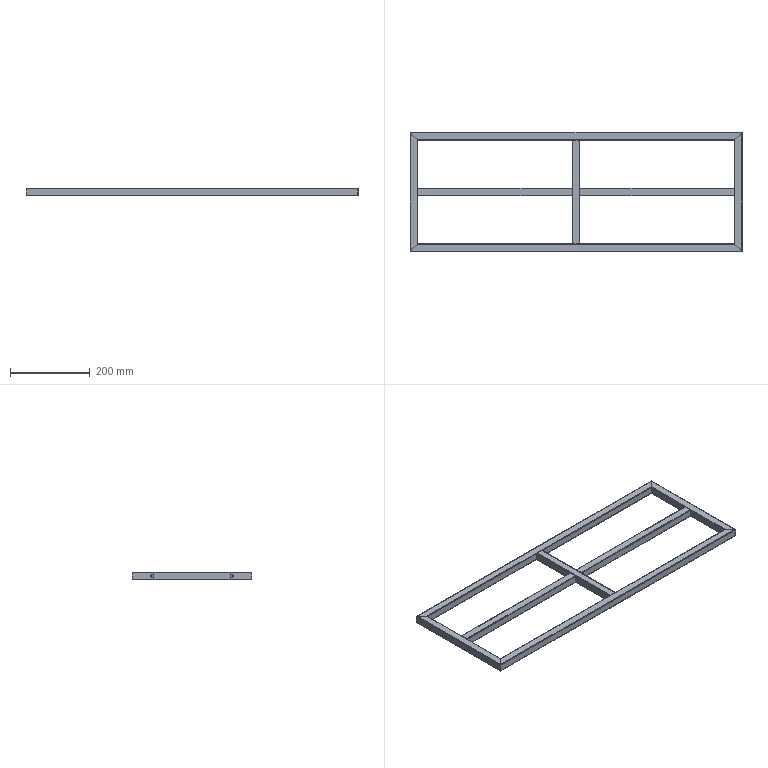Part | SolidWorks | features Cut 2, WeldMemberFeat 1, WeldmentFeature 1 | 7 solids | 142 faces | box 835 x 300 x 20 mm | volume 284675 mm3 | cylinder 72 | plane 70 | commonest cylinder face diameters 0.6 x28 3 x28 7 x16